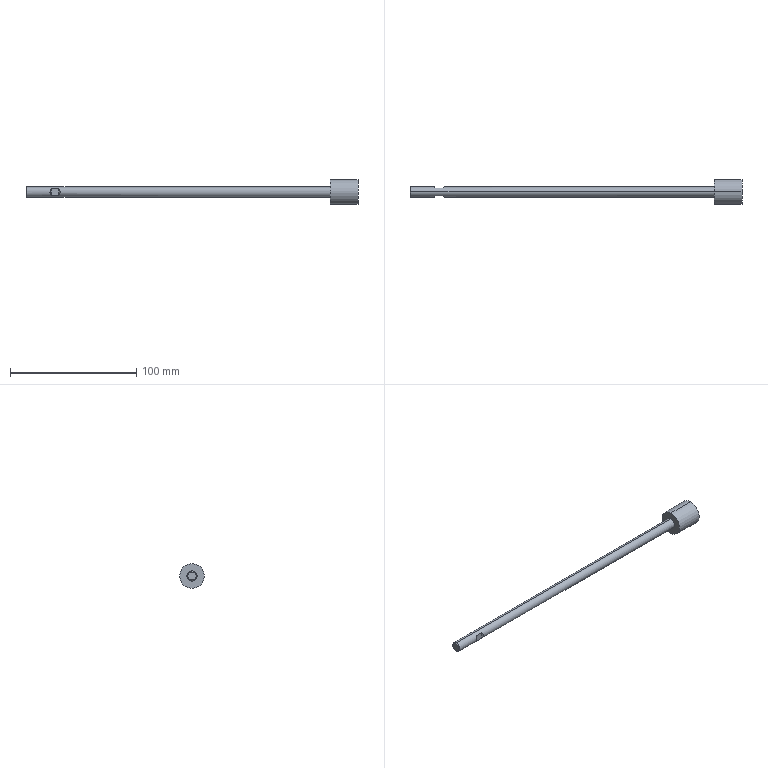Part | SolidWorks | features BaseBody 1 | 1 solid | 15 faces | box 263 x 19.5 x 19.5 mm | volume 18628 mm3 | plane 9 | cylinder 4 | cone 2 | commonest cylinder face diameters 8 x2 19.5 x2
STEP:
#1=CARTESIAN_POINT('',(-5.,-3.,-2.646));
#2=VERTEX_POINT('',#1);
#3=CARTESIAN_POINT('',(-5.,-3.,2.646));
#4=VERTEX_POINT('',#3);
#5=CARTESIAN_POINT('',(-5.,-3.,-2.646));
#6=CARTESIAN_POINT('',(-3.6,-4.4,-1.058));
#7=CARTESIAN_POINT('',(-3.6,-4.4,1.058));
#8=CARTESIAN_POINT('',(-5.,-3.,2.646));
#9=(BOUNDED_CURVE()B_SPLINE_CURVE(3,(#5,#6,#7,#8),.UNSPECIFIED.,.F.,.F.)B_SPLINE_CURVE_WITH_KNOTS((4,4),(5.56,7.006),.UNSPECIFIED.)CURVE()GEOMETRIC_REPRESENTATION_ITEM()RATIONAL_B_SPLINE_CURVE((1.,0.8333,0.8333,1.))REPRESENTATION_ITEM(''));
#10=EDGE_CURVE('',#2,#4,#9,.T.);
#11=ORIENTED_EDGE('',*,*,#10,.F.);
#12=CARTESIAN_POINT('',(-11.,-3.,-2.646));
#13=VERTEX_POINT('',#12);
#14=CARTESIAN_POINT('',(232.,-3.,-2.646));
#15=DIRECTION('',(1.,0.,0.));
#16=VECTOR('',#15,1000.);
#17=LINE('',#14,#16);
#18=EDGE_CURVE('',#13,#2,#17,.T.);
#19=ORIENTED_EDGE('',*,*,#18,.F.);
#20=CARTESIAN_POINT('',(-11.,-3.,2.646));
#21=VERTEX_POINT('',#20);
#22=CARTESIAN_POINT('',(-11.,-3.,2.646));
#23=CARTESIAN_POINT('',(-12.4,-4.4,1.058));
#24=CARTESIAN_POINT('',(-12.4,-4.4,-1.058));
#25=CARTESIAN_POINT('',(-11.,-3.,-2.646));
#26=(BOUNDED_CURVE()B_SPLINE_CURVE(3,(#22,#23,#24,#25),.UNSPECIFIED.,.F.,.F.)B_SPLINE_CURVE_WITH_KNOTS((4,4),(2.419,3.864),.UNSPECIFIED.)CURVE()GEOMETRIC_REPRESENTATION_ITEM()RATIONAL_B_SPLINE_CURVE((1.,0.8333,0.8333,1.))REPRESENTATION_ITEM(''));
#27=EDGE_CURVE('',#21,#13,#26,.T.);
#28=ORIENTED_EDGE('',*,*,#27,.F.);
#29=CARTESIAN_POINT('',(232.,-3.,2.646));
#30=DIRECTION('',(-1.,0.,0.));
#31=VECTOR('',#30,1000.);
#32=LINE('',#29,#31);
#33=EDGE_CURVE('',#4,#21,#32,.T.);
#34=ORIENTED_EDGE('',*,*,#33,.F.);
#35=EDGE_LOOP('',(#11,#19,#28,#34));
#36=FACE_BOUND('',#35,.T.);
#37=CARTESIAN_POINT('',(210.,0.,4.));
#38=VERTEX_POINT('',#37);
#39=CARTESIAN_POINT('',(210.,0.,-4.));
#40=VERTEX_POINT('',#39);
#41=CARTESIAN_POINT('',(210.,0.,0.));
#42=DIRECTION('',(1.,0.,0.));
#43=DIRECTION('',(0.,0.,-1.));
#44=AXIS2_PLACEMENT_3D('',#41,#42,#43);
#45=CIRCLE('',#44,4.);
#46=EDGE_CURVE('',#38,#40,#45,.T.);
#47=ORIENTED_EDGE('',*,*,#46,.F.);
#48=CARTESIAN_POINT('',(-30.233,0.,4.));
#49=VERTEX_POINT('',#48);
#50=CARTESIAN_POINT('',(232.,0.,4.));
#51=DIRECTION('',(-1.,0.,0.));
#52=VECTOR('',#51,1000.);
#53=LINE('',#50,#52);
#54=EDGE_CURVE('',#38,#49,#53,.T.);
#55=ORIENTED_EDGE('',*,*,#54,.T.);
#56=CARTESIAN_POINT('',(-30.233,0.,-4.));
#57=VERTEX_POINT('',#56);
#58=CARTESIAN_POINT('',(-30.233,0.,0.));
#59=DIRECTION('',(1.,0.,0.));
#60=DIRECTION('',(0.,0.,-1.));
#61=AXIS2_PLACEMENT_3D('',#58,#59,#60);
#62=CIRCLE('',#61,4.);
#63=EDGE_CURVE('',#49,#57,#62,.T.);
#64=ORIENTED_EDGE('',*,*,#63,.T.);
#65=CARTESIAN_POINT('',(232.,0.,-4.));
#66=DIRECTION('',(-1.,0.,0.));
#67=VECTOR('',#66,1000.);
#68=LINE('',#65,#67);
#69=EDGE_CURVE('',#40,#57,#68,.T.);
#70=ORIENTED_EDGE('',*,*,#69,.F.);
#71=EDGE_LOOP('',(#47,#55,#64,#70));
#72=FACE_OUTER_BOUND('',#71,.T.);
#73=CARTESIAN_POINT('',(232.,0.,0.));
#74=DIRECTION('',(-1.,0.,0.));
#75=DIRECTION('',(0.,0.,-1.));
#76=AXIS2_PLACEMENT_3D('',#73,#74,#75);
#77=CYLINDRICAL_SURFACE('',#76,4.);
#78=ADVANCED_FACE('',(#36,#72),#77,.T.);
#79=CARTESIAN_POINT('',(232.,0.,9.75));
#80=VERTEX_POINT('',#79);
#81=CARTESIAN_POINT('',(232.,0.,-9.75));
#82=VERTEX_POINT('',#81);
#83=CARTESIAN_POINT('',(232.,0.,0.));
#84=DIRECTION('',(1.,0.,0.));
#85=DIRECTION('',(0.,0.,-1.));
#86=AXIS2_PLACEMENT_3D('',#83,#84,#85);
#87=CIRCLE('',#86,9.75);
#88=EDGE_CURVE('',#80,#82,#87,.T.);
#89=ORIENTED_EDGE('',*,*,#88,.F.);
#90=CARTESIAN_POINT('',(210.,0.,9.75));
#91=VERTEX_POINT('',#90);
#92=CARTESIAN_POINT('',(232.,0.,9.75));
#93=DIRECTION('',(-1.,0.,0.));
#94=VECTOR('',#93,1000.);
#95=LINE('',#92,#94);
#96=EDGE_CURVE('',#80,#91,#95,.T.);
#97=ORIENTED_EDGE('',*,*,#96,.T.);
#98=CARTESIAN_POINT('',(210.,0.,-9.75));
#99=VERTEX_POINT('',#98);
#100=CARTESIAN_POINT('',(210.,0.,0.));
#101=DIRECTION('',(1.,0.,0.));
#102=DIRECTION('',(0.,0.,-1.));
#103=AXIS2_PLACEMENT_3D('',#100,#101,#102);
#104=CIRCLE('',#103,9.75);
#105=EDGE_CURVE('',#91,#99,#104,.T.);
#106=ORIENTED_EDGE('',*,*,#105,.T.);
#107=CARTESIAN_POINT('',(232.,0.,-9.75));
#108=DIRECTION('',(-1.,0.,0.));
#109=VECTOR('',#108,1000.);
#110=LINE('',#107,#109);
#111=EDGE_CURVE('',#82,#99,#110,.T.);
#112=ORIENTED_EDGE('',*,*,#111,.F.);
#113=EDGE_LOOP('',(#89,#97,#106,#112));
#114=FACE_OUTER_BOUND('',#113,.T.);
#115=CARTESIAN_POINT('',(232.,0.,0.));
#116=DIRECTION('',(-1.,0.,0.));
#117=DIRECTION('',(0.,0.,-1.));
#118=AXIS2_PLACEMENT_3D('',#115,#116,#117);
#119=CYLINDRICAL_SURFACE('',#118,9.75);
#120=ADVANCED_FACE('',(#114),#119,.T.);
#121=CARTESIAN_POINT('',(-31.,0.,-3.233));
#122=VERTEX_POINT('',#121);
#123=CARTESIAN_POINT('',(-31.,0.,3.233));
#124=VERTEX_POINT('',#123);
#125=CARTESIAN_POINT('',(-31.,0.,0.));
#126=DIRECTION('',(1.,0.,0.));
#127=DIRECTION('',(0.,0.,-1.));
#128=AXIS2_PLACEMENT_3D('',#125,#126,#127);
#129=CIRCLE('',#128,3.233);
#130=EDGE_CURVE('',#122,#124,#129,.T.);
#131=ORIENTED_EDGE('',*,*,#130,.T.);
#132=CARTESIAN_POINT('',(-31.,0.,3.233));
#133=DIRECTION('',(0.7071,0.,0.7071));
#134=VECTOR('',#133,1000.);
#135=LINE('',#132,#134);
#136=EDGE_CURVE('',#124,#49,#135,.T.);
#137=ORIENTED_EDGE('',*,*,#136,.T.);
#138=CARTESIAN_POINT('',(-30.233,0.,0.));
#139=DIRECTION('',(1.,0.,0.));
#140=DIRECTION('',(0.,0.,-1.));
#141=AXIS2_PLACEMENT_3D('',#138,#139,#140);
#142=CIRCLE('',#141,4.);
#143=EDGE_CURVE('',#57,#49,#142,.T.);
#144=ORIENTED_EDGE('',*,*,#143,.F.);
#145=CARTESIAN_POINT('',(-31.,0.,-3.233));
#146=DIRECTION('',(0.7071,0.,-0.7071));
#147=VECTOR('',#146,1000.);
#148=LINE('',#145,#147);
#149=EDGE_CURVE('',#122,#57,#148,.T.);
#150=ORIENTED_EDGE('',*,*,#149,.F.);
#151=EDGE_LOOP('',(#131,#137,#144,#150));
#152=FACE_OUTER_BOUND('',#151,.T.);
#153=CARTESIAN_POINT('',(-31.,0.,0.));
#154=DIRECTION('',(1.,0.,0.));
#155=DIRECTION('',(0.,0.,-1.));
#156=AXIS2_PLACEMENT_3D('',#153,#154,#155);
#157=CONICAL_SURFACE('',#156,3.233,0.7854);
#158=ADVANCED_FACE('',(#152),#157,.T.);
#159=CARTESIAN_POINT('',(-5.,3.,2.646));
#160=VERTEX_POINT('',#159);
#161=CARTESIAN_POINT('',(-5.,3.,-2.646));
#162=VERTEX_POINT('',#161);
#163=CARTESIAN_POINT('',(-5.,3.,8.));
#164=DIRECTION('',(0.,0.,-1.));
#165=VECTOR('',#164,1000.);
#166=LINE('',#163,#165);
#167=EDGE_CURVE('',#160,#162,#166,.T.);
#168=ORIENTED_EDGE('',*,*,#167,.F.);
#169=CARTESIAN_POINT('',(-5.,3.,2.646));
#170=CARTESIAN_POINT('',(-3.6,4.4,1.058));
#171=CARTESIAN_POINT('',(-3.6,4.4,-1.058));
#172=CARTESIAN_POINT('',(-5.,3.,-2.646));
#173=(BOUNDED_CURVE()B_SPLINE_CURVE(3,(#169,#170,#171,#172),.UNSPECIFIED.,.F.,.F.)B_SPLINE_CURVE_WITH_KNOTS((4,4),(5.56,7.006),.UNSPECIFIED.)CURVE()GEOMETRIC_REPRESENTATION_ITEM()RATIONAL_B_SPLINE_CURVE((1.,0.8333,0.8333,1.))REPRESENTATION_ITEM(''));
#174=EDGE_CURVE('',#160,#162,#173,.T.);
#175=ORIENTED_EDGE('',*,*,#174,.T.);
#176=EDGE_LOOP('',(#168,#175));
#177=FACE_OUTER_BOUND('',#176,.T.);
#178=CARTESIAN_POINT('',(-5.,3.,8.));
#179=DIRECTION('',(-0.7071,0.7071,0.));
#180=DIRECTION('',(0.,0.,1.));
#181=AXIS2_PLACEMENT_3D('',#178,#179,#180);
#182=PLANE('',#181);
#183=ADVANCED_FACE('',(#177),#182,.T.);
#184=CARTESIAN_POINT('',(-11.,3.,2.646));
#185=VERTEX_POINT('',#184);
#186=CARTESIAN_POINT('',(232.,3.,2.646));
#187=DIRECTION('',(1.,0.,0.));
#188=VECTOR('',#187,1000.);
#189=LINE('',#186,#188);
#190=EDGE_CURVE('',#185,#160,#189,.T.);
#191=ORIENTED_EDGE('',*,*,#190,.T.);
#192=ORIENTED_EDGE('',*,*,#167,.T.);
#193=CARTESIAN_POINT('',(-11.,3.,-2.646));
#194=VERTEX_POINT('',#193);
#195=CARTESIAN_POINT('',(232.,3.,-2.646));
#196=DIRECTION('',(-1.,0.,0.));
#197=VECTOR('',#196,1000.);
#198=LINE('',#195,#197);
#199=EDGE_CURVE('',#162,#194,#198,.T.);
#200=ORIENTED_EDGE('',*,*,#199,.T.);
#201=CARTESIAN_POINT('',(-11.,3.,8.));
#202=DIRECTION('',(0.,0.,-1.));
#203=VECTOR('',#202,1000.);
#204=LINE('',#201,#203);
#205=EDGE_CURVE('',#185,#194,#204,.T.);
#206=ORIENTED_EDGE('',*,*,#205,.F.);
#207=EDGE_LOOP('',(#191,#192,#200,#206));
#208=FACE_OUTER_BOUND('',#207,.T.);
#209=CARTESIAN_POINT('',(-11.,3.,8.));
#210=DIRECTION('',(0.,1.,0.));
#211=DIRECTION('',(1.,0.,0.));
#212=AXIS2_PLACEMENT_3D('',#209,#210,#211);
#213=PLANE('',#212);
#214=ADVANCED_FACE('',(#208),#213,.T.);
#215=ORIENTED_EDGE('',*,*,#205,.T.);
#216=CARTESIAN_POINT('',(-11.,3.,-2.646));
#217=CARTESIAN_POINT('',(-12.4,4.4,-1.058));
#218=CARTESIAN_POINT('',(-12.4,4.4,1.058));
#219=CARTESIAN_POINT('',(-11.,3.,2.646));
#220=(BOUNDED_CURVE()B_SPLINE_CURVE(3,(#216,#217,#218,#219),.UNSPECIFIED.,.F.,.F.)B_SPLINE_CURVE_WITH_KNOTS((4,4),(2.419,3.864),.UNSPECIFIED.)CURVE()GEOMETRIC_REPRESENTATION_ITEM()RATIONAL_B_SPLINE_CURVE((1.,0.8333,0.8333,1.))REPRESENTATION_ITEM(''));
#221=EDGE_CURVE('',#194,#185,#220,.T.);
#222=ORIENTED_EDGE('',*,*,#221,.T.);
#223=EDGE_LOOP('',(#215,#222));
#224=FACE_OUTER_BOUND('',#223,.T.);
#225=CARTESIAN_POINT('',(-13.,5.,8.));
#226=DIRECTION('',(0.7071,0.7071,0.));
#227=DIRECTION('',(0.,0.,-1.));
#228=AXIS2_PLACEMENT_3D('',#225,#226,#227);
#229=PLANE('',#228);
#230=ADVANCED_FACE('',(#224),#229,.T.);
#231=ORIENTED_EDGE('',*,*,#10,.T.);
#232=CARTESIAN_POINT('',(-5.,-3.,8.));
#233=DIRECTION('',(0.,0.,-1.));
#234=VECTOR('',#233,1000.);
#235=LINE('',#232,#234);
#236=EDGE_CURVE('',#4,#2,#235,.T.);
#237=ORIENTED_EDGE('',*,*,#236,.T.);
#238=EDGE_LOOP('',(#231,#237));
#239=FACE_OUTER_BOUND('',#238,.T.);
#240=CARTESIAN_POINT('',(-1.,-7.,8.));
#241=DIRECTION('',(-0.7071,-0.7071,0.));
#242=DIRECTION('',(-0.7071,0.7071,0.));
#243=AXIS2_PLACEMENT_3D('',#240,#241,#242);
#244=PLANE('',#243);
#245=ADVANCED_FACE('',(#239),#244,.T.);
#246=ORIENTED_EDGE('',*,*,#136,.F.);
#247=CARTESIAN_POINT('',(-31.,0.,0.));
#248=DIRECTION('',(1.,0.,0.));
#249=DIRECTION('',(0.,0.,-1.));
#250=AXIS2_PLACEMENT_3D('',#247,#248,#249);
#251=CIRCLE('',#250,3.233);
#252=EDGE_CURVE('',#124,#122,#251,.T.);
#253=ORIENTED_EDGE('',*,*,#252,.T.);
#254=ORIENTED_EDGE('',*,*,#149,.T.);
#255=ORIENTED_EDGE('',*,*,#63,.F.);
#256=EDGE_LOOP('',(#246,#253,#254,#255));
#257=FACE_OUTER_BOUND('',#256,.T.);
#258=CARTESIAN_POINT('',(-31.,0.,0.));
#259=DIRECTION('',(1.,0.,0.));
#260=DIRECTION('',(0.,0.,-1.));
#261=AXIS2_PLACEMENT_3D('',#258,#259,#260);
#262=CONICAL_SURFACE('',#261,3.233,0.7854);
#263=ADVANCED_FACE('',(#257),#262,.T.);
#264=ORIENTED_EDGE('',*,*,#130,.F.);
#265=ORIENTED_EDGE('',*,*,#252,.F.);
#266=EDGE_LOOP('',(#264,#265));
#267=FACE_OUTER_BOUND('',#266,.T.);
#268=CARTESIAN_POINT('',(-31.,0.,0.));
#269=DIRECTION('',(1.,0.,0.));
#270=DIRECTION('',(0.,1.,0.));
#271=AXIS2_PLACEMENT_3D('',#268,#269,#270);
#272=PLANE('',#271);
#273=ADVANCED_FACE('',(#267),#272,.F.);
#274=CARTESIAN_POINT('',(232.,0.,0.));
#275=DIRECTION('',(1.,0.,0.));
#276=DIRECTION('',(0.,0.,-1.));
#277=AXIS2_PLACEMENT_3D('',#274,#275,#276);
#278=CIRCLE('',#277,9.75);
#279=EDGE_CURVE('',#82,#80,#278,.T.);
#280=ORIENTED_EDGE('',*,*,#279,.T.);
#281=ORIENTED_EDGE('',*,*,#88,.T.);
#282=EDGE_LOOP('',(#280,#281));
#283=FACE_OUTER_BOUND('',#282,.T.);
#284=CARTESIAN_POINT('',(232.,9.75,0.));
#285=DIRECTION('',(-1.,0.,0.));
#286=DIRECTION('',(0.,0.,1.));
#287=AXIS2_PLACEMENT_3D('',#284,#285,#286);
#288=PLANE('',#287);
#289=ADVANCED_FACE('',(#283),#288,.F.);
#290=ORIENTED_EDGE('',*,*,#96,.F.);
#291=ORIENTED_EDGE('',*,*,#279,.F.);
#292=ORIENTED_EDGE('',*,*,#111,.T.);
#293=CARTESIAN_POINT('',(210.,0.,0.));
#294=DIRECTION('',(1.,0.,0.));
#295=DIRECTION('',(0.,0.,-1.));
#296=AXIS2_PLACEMENT_3D('',#293,#294,#295);
#297=CIRCLE('',#296,9.75);
#298=EDGE_CURVE('',#99,#91,#297,.T.);
#299=ORIENTED_EDGE('',*,*,#298,.T.);
#300=EDGE_LOOP('',(#290,#291,#292,#299));
#301=FACE_OUTER_BOUND('',#300,.T.);
#302=CARTESIAN_POINT('',(232.,0.,0.));
#303=DIRECTION('',(-1.,0.,0.));
#304=DIRECTION('',(0.,0.,-1.));
#305=AXIS2_PLACEMENT_3D('',#302,#303,#304);
#306=CYLINDRICAL_SURFACE('',#305,9.75);
#307=ADVANCED_FACE('',(#301),#306,.T.);
#308=CARTESIAN_POINT('',(210.,0.,0.));
#309=DIRECTION('',(1.,0.,0.));
#310=DIRECTION('',(0.,0.,-1.));
#311=AXIS2_PLACEMENT_3D('',#308,#309,#310);
#312=CIRCLE('',#311,4.);
#313=EDGE_CURVE('',#40,#38,#312,.T.);
#314=ORIENTED_EDGE('',*,*,#313,.T.);
#315=ORIENTED_EDGE('',*,*,#46,.T.);
#316=EDGE_LOOP('',(#314,#315));
#317=FACE_BOUND('',#316,.T.);
#318=ORIENTED_EDGE('',*,*,#298,.F.);
#319=ORIENTED_EDGE('',*,*,#105,.F.);
#320=EDGE_LOOP('',(#318,#319));
#321=FACE_OUTER_BOUND('',#320,.T.);
#322=CARTESIAN_POINT('',(210.,4.,0.));
#323=DIRECTION('',(1.,0.,0.));
#324=DIRECTION('',(0.,1.,0.));
#325=AXIS2_PLACEMENT_3D('',#322,#323,#324);
#326=PLANE('',#325);
#327=ADVANCED_FACE('',(#317,#321),#326,.F.);
#328=ORIENTED_EDGE('',*,*,#54,.F.);
#329=ORIENTED_EDGE('',*,*,#313,.F.);
#330=ORIENTED_EDGE('',*,*,#69,.T.);
#331=ORIENTED_EDGE('',*,*,#143,.T.);
#332=EDGE_LOOP('',(#328,#329,#330,#331));
#333=FACE_OUTER_BOUND('',#332,.T.);
#334=ORIENTED_EDGE('',*,*,#221,.F.);
#335=ORIENTED_EDGE('',*,*,#199,.F.);
#336=ORIENTED_EDGE('',*,*,#174,.F.);
#337=ORIENTED_EDGE('',*,*,#190,.F.);
#338=EDGE_LOOP('',(#334,#335,#336,#337));
#339=FACE_BOUND('',#338,.T.);
#340=CARTESIAN_POINT('',(232.,0.,0.));
#341=DIRECTION('',(-1.,0.,0.));
#342=DIRECTION('',(0.,0.,-1.));
#343=AXIS2_PLACEMENT_3D('',#340,#341,#342);
#344=CYLINDRICAL_SURFACE('',#343,4.);
#345=ADVANCED_FACE('',(#333,#339),#344,.T.);
#346=ORIENTED_EDGE('',*,*,#18,.T.);
#347=ORIENTED_EDGE('',*,*,#236,.F.);
#348=ORIENTED_EDGE('',*,*,#33,.T.);
#349=CARTESIAN_POINT('',(-11.,-3.,8.));
#350=DIRECTION('',(0.,0.,-1.));
#351=VECTOR('',#350,1000.);
#352=LINE('',#349,#351);
#353=EDGE_CURVE('',#21,#13,#352,.T.);
#354=ORIENTED_EDGE('',*,*,#353,.T.);
#355=EDGE_LOOP('',(#346,#347,#348,#354));
#356=FACE_OUTER_BOUND('',#355,.T.);
#357=CARTESIAN_POINT('',(-5.,-3.,8.));
#358=DIRECTION('',(0.,-1.,0.));
#359=DIRECTION('',(0.,0.,-1.));
#360=AXIS2_PLACEMENT_3D('',#357,#358,#359);
#361=PLANE('',#360);
#362=ADVANCED_FACE('',(#356),#361,.T.);
#363=ORIENTED_EDGE('',*,*,#27,.T.);
#364=ORIENTED_EDGE('',*,*,#353,.F.);
#365=EDGE_LOOP('',(#363,#364));
#366=FACE_OUTER_BOUND('',#365,.T.);
#367=CARTESIAN_POINT('',(-11.,-3.,8.));
#368=DIRECTION('',(0.7071,-0.7071,0.));
#369=DIRECTION('',(0.,0.,-1.));
#370=AXIS2_PLACEMENT_3D('',#367,#368,#369);
#371=PLANE('',#370);
#372=ADVANCED_FACE('',(#366),#371,.T.);
#373=CLOSED_SHELL('',(#78,#120,#158,#183,#214,#230,#245,#263,#273,#289,#307,#327,#345,#362,#372));
#374=MANIFOLD_SOLID_BREP('',#373);
#375=CARTESIAN_POINT('',(0.,0.,0.));
#376=DIRECTION('',(0.,0.,1.));
#377=DIRECTION('',(1.,0.,0.));
#378=AXIS2_PLACEMENT_3D('',#375,#376,#377);
#379=(LENGTH_UNIT()NAMED_UNIT(*)SI_UNIT(.MILLI.,.METRE.));
#380=UNCERTAINTY_MEASURE_WITH_UNIT(LENGTH_MEASURE(0.00001),#379,'','');
#381=(NAMED_UNIT(*)PLANE_ANGLE_UNIT()SI_UNIT($,.RADIAN.));
#382=(NAMED_UNIT(*)SI_UNIT($,.STERADIAN.)SOLID_ANGLE_UNIT());
#383=(GEOMETRIC_REPRESENTATION_CONTEXT(3)GLOBAL_UNCERTAINTY_ASSIGNED_CONTEXT((#380))GLOBAL_UNIT_ASSIGNED_CONTEXT((#379,#381,#382))REPRESENTATION_CONTEXT('',''));
#384=ADVANCED_BREP_SHAPE_REPRESENTATION('',(#374,#378),#383);